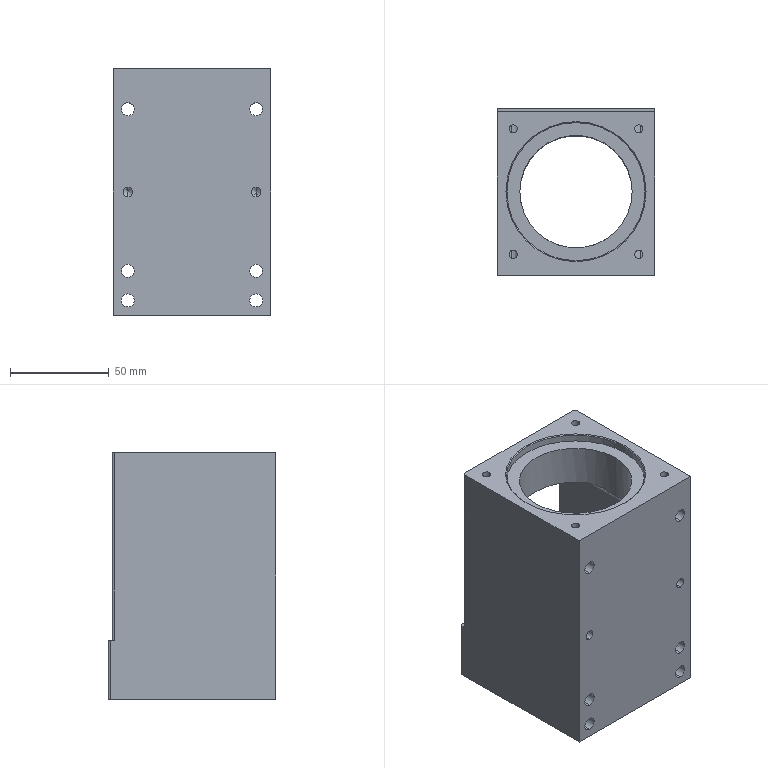Part | STEP file | 1 solid | 109 faces | box 80 x 85 x 125 mm | volume 372147 mm3 | cylinder 66 | cone 22 | plane 21 | commonest cylinder face diameters 5 x12 6.6 x12 11 x12 3.3 x8 4.2 x8 2 x4